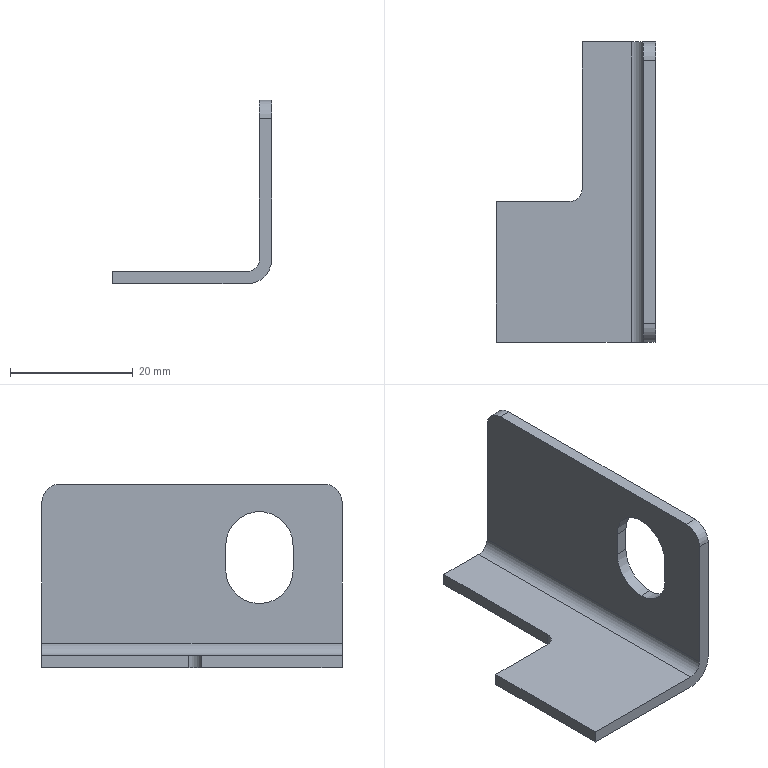Part | STEP file | 750038334 | 1 solid | 20 faces | box 26 x 49 x 30 mm | volume 4154 mm3 | plane 12 | cylinder 8 | commonest cylinder face diameters 11 x3 4 x2 6 x2 8 x1
STEP:
#1=CARTESIAN_POINT('',(24.,71.5,10.5));
#2=VERTEX_POINT('',#1);
#3=CARTESIAN_POINT('',(24.,77.,16.));
#4=VERTEX_POINT('',#3);
#5=CARTESIAN_POINT('',(24.,71.5,16.));
#6=DIRECTION('',(1.,0.,0.));
#7=DIRECTION('',(0.,0.,-1.));
#8=AXIS2_PLACEMENT_3D('',#5,#6,#7);
#9=CIRCLE('',#8,5.5);
#10=EDGE_CURVE('',#2,#4,#9,.T.);
#11=ORIENTED_EDGE('',*,*,#10,.F.);
#12=CARTESIAN_POINT('',(26.,71.5,10.5));
#13=VERTEX_POINT('',#12);
#14=CARTESIAN_POINT('',(-37.063,71.5,10.5));
#15=DIRECTION('',(1.,0.,0.));
#16=VECTOR('',#15,1000.);
#17=LINE('',#14,#16);
#18=EDGE_CURVE('',#2,#13,#17,.T.);
#19=ORIENTED_EDGE('',*,*,#18,.T.);
#20=CARTESIAN_POINT('',(26.,77.,16.));
#21=VERTEX_POINT('',#20);
#22=CARTESIAN_POINT('',(26.,71.5,16.));
#23=DIRECTION('',(-1.,0.,0.));
#24=DIRECTION('',(0.,0.,-1.));
#25=AXIS2_PLACEMENT_3D('',#22,#23,#24);
#26=CIRCLE('',#25,5.5);
#27=EDGE_CURVE('',#21,#13,#26,.T.);
#28=ORIENTED_EDGE('',*,*,#27,.F.);
#29=CARTESIAN_POINT('',(-37.063,77.,16.));
#30=DIRECTION('',(-1.,0.,0.));
#31=VECTOR('',#30,1000.);
#32=LINE('',#29,#31);
#33=EDGE_CURVE('',#21,#4,#32,.T.);
#34=ORIENTED_EDGE('',*,*,#33,.T.);
#35=EDGE_LOOP('',(#11,#19,#28,#34));
#36=FACE_OUTER_BOUND('',#35,.T.);
#37=CARTESIAN_POINT('',(-37.063,71.5,16.));
#38=DIRECTION('',(1.,0.,0.));
#39=DIRECTION('',(0.,0.,-1.));
#40=AXIS2_PLACEMENT_3D('',#37,#38,#39);
#41=CYLINDRICAL_SURFACE('',#40,5.5);
#42=ADVANCED_FACE('',(#36),#41,.F.);
#43=CARTESIAN_POINT('',(24.,107.,27.));
#44=VERTEX_POINT('',#43);
#45=CARTESIAN_POINT('',(24.,107.,4.));
#46=VERTEX_POINT('',#45);
#47=CARTESIAN_POINT('',(24.,107.,4.));
#48=DIRECTION('',(0.,0.,-1.));
#49=VECTOR('',#48,1000.);
#50=LINE('',#47,#49);
#51=EDGE_CURVE('',#44,#46,#50,.T.);
#52=ORIENTED_EDGE('',*,*,#51,.T.);
#53=CARTESIAN_POINT('',(24.,58.,4.));
#54=VERTEX_POINT('',#53);
#55=CARTESIAN_POINT('',(24.,58.,4.));
#56=DIRECTION('',(0.,-1.,0.));
#57=VECTOR('',#56,1000.);
#58=LINE('',#55,#57);
#59=EDGE_CURVE('',#46,#54,#58,.T.);
#60=ORIENTED_EDGE('',*,*,#59,.T.);
#61=CARTESIAN_POINT('',(24.,58.,27.));
#62=VERTEX_POINT('',#61);
#63=CARTESIAN_POINT('',(24.,58.,4.));
#64=DIRECTION('',(0.,0.,1.));
#65=VECTOR('',#64,1000.);
#66=LINE('',#63,#65);
#67=EDGE_CURVE('',#54,#62,#66,.T.);
#68=ORIENTED_EDGE('',*,*,#67,.T.);
#69=CARTESIAN_POINT('',(24.,61.,30.));
#70=VERTEX_POINT('',#69);
#71=CARTESIAN_POINT('',(24.,61.,27.));
#72=DIRECTION('',(-1.,0.,0.));
#73=DIRECTION('',(0.,1.,0.));
#74=AXIS2_PLACEMENT_3D('',#71,#72,#73);
#75=CIRCLE('',#74,3.);
#76=EDGE_CURVE('',#62,#70,#75,.T.);
#77=ORIENTED_EDGE('',*,*,#76,.T.);
#78=CARTESIAN_POINT('',(24.,104.,30.));
#79=VERTEX_POINT('',#78);
#80=CARTESIAN_POINT('',(24.,58.,30.));
#81=DIRECTION('',(0.,1.,0.));
#82=VECTOR('',#81,1000.);
#83=LINE('',#80,#82);
#84=EDGE_CURVE('',#70,#79,#83,.T.);
#85=ORIENTED_EDGE('',*,*,#84,.T.);
#86=CARTESIAN_POINT('',(24.,104.,27.));
#87=DIRECTION('',(-1.,0.,0.));
#88=DIRECTION('',(0.,0.,-1.));
#89=AXIS2_PLACEMENT_3D('',#86,#87,#88);
#90=CIRCLE('',#89,3.);
#91=EDGE_CURVE('',#79,#44,#90,.T.);
#92=ORIENTED_EDGE('',*,*,#91,.T.);
#93=EDGE_LOOP('',(#52,#60,#68,#77,#85,#92));
#94=FACE_OUTER_BOUND('',#93,.T.);
#95=CARTESIAN_POINT('',(24.,66.,16.));
#96=VERTEX_POINT('',#95);
#97=CARTESIAN_POINT('',(24.,71.5,16.));
#98=DIRECTION('',(1.,0.,0.));
#99=DIRECTION('',(0.,0.,-1.));
#100=AXIS2_PLACEMENT_3D('',#97,#98,#99);
#101=CIRCLE('',#100,5.5);
#102=EDGE_CURVE('',#96,#2,#101,.T.);
#103=ORIENTED_EDGE('',*,*,#102,.T.);
#104=ORIENTED_EDGE('',*,*,#10,.T.);
#105=CARTESIAN_POINT('',(24.,77.,20.));
#106=VERTEX_POINT('',#105);
#107=CARTESIAN_POINT('',(24.,77.,4.));
#108=DIRECTION('',(0.,0.,1.));
#109=VECTOR('',#108,1000.);
#110=LINE('',#107,#109);
#111=EDGE_CURVE('',#4,#106,#110,.T.);
#112=ORIENTED_EDGE('',*,*,#111,.T.);
#113=CARTESIAN_POINT('',(24.,66.,20.));
#114=VERTEX_POINT('',#113);
#115=CARTESIAN_POINT('',(24.,71.5,20.));
#116=DIRECTION('',(1.,0.,0.));
#117=DIRECTION('',(0.,0.,-1.));
#118=AXIS2_PLACEMENT_3D('',#115,#116,#117);
#119=CIRCLE('',#118,5.5);
#120=EDGE_CURVE('',#106,#114,#119,.T.);
#121=ORIENTED_EDGE('',*,*,#120,.T.);
#122=CARTESIAN_POINT('',(24.,66.,4.));
#123=DIRECTION('',(0.,0.,-1.));
#124=VECTOR('',#123,1000.);
#125=LINE('',#122,#124);
#126=EDGE_CURVE('',#114,#96,#125,.T.);
#127=ORIENTED_EDGE('',*,*,#126,.T.);
#128=EDGE_LOOP('',(#103,#104,#112,#121,#127));
#129=FACE_BOUND('',#128,.T.);
#130=CARTESIAN_POINT('',(24.,58.,4.));
#131=DIRECTION('',(-1.,0.,0.));
#132=DIRECTION('',(0.,-1.,0.));
#133=AXIS2_PLACEMENT_3D('',#130,#131,#132);
#134=PLANE('',#133);
#135=ADVANCED_FACE('',(#94,#129),#134,.T.);
#136=CARTESIAN_POINT('',(22.,58.,2.));
#137=VERTEX_POINT('',#136);
#138=CARTESIAN_POINT('',(22.,107.,2.));
#139=VERTEX_POINT('',#138);
#140=CARTESIAN_POINT('',(22.,58.,2.));
#141=DIRECTION('',(0.,1.,0.));
#142=VECTOR('',#141,1000.);
#143=LINE('',#140,#142);
#144=EDGE_CURVE('',#137,#139,#143,.T.);
#145=ORIENTED_EDGE('',*,*,#144,.F.);
#146=CARTESIAN_POINT('',(22.,58.,4.));
#147=DIRECTION('',(0.,1.,0.));
#148=DIRECTION('',(-1.,0.,0.));
#149=AXIS2_PLACEMENT_3D('',#146,#147,#148);
#150=CIRCLE('',#149,2.);
#151=EDGE_CURVE('',#54,#137,#150,.T.);
#152=ORIENTED_EDGE('',*,*,#151,.F.);
#153=ORIENTED_EDGE('',*,*,#59,.F.);
#154=CARTESIAN_POINT('',(22.,107.,4.));
#155=DIRECTION('',(0.,-1.,0.));
#156=DIRECTION('',(-1.,0.,0.));
#157=AXIS2_PLACEMENT_3D('',#154,#155,#156);
#158=CIRCLE('',#157,2.);
#159=EDGE_CURVE('',#139,#46,#158,.T.);
#160=ORIENTED_EDGE('',*,*,#159,.F.);
#161=EDGE_LOOP('',(#145,#152,#153,#160));
#162=FACE_OUTER_BOUND('',#161,.T.);
#163=CARTESIAN_POINT('',(22.,58.,4.));
#164=DIRECTION('',(0.,1.,0.));
#165=DIRECTION('',(-1.,0.,0.));
#166=AXIS2_PLACEMENT_3D('',#163,#164,#165);
#167=CYLINDRICAL_SURFACE('',#166,2.);
#168=ADVANCED_FACE('',(#162),#167,.F.);
#169=CARTESIAN_POINT('',(14.,107.,2.));
#170=VERTEX_POINT('',#169);
#171=CARTESIAN_POINT('',(14.,107.,2.));
#172=DIRECTION('',(1.,0.,0.));
#173=VECTOR('',#172,1000.);
#174=LINE('',#171,#173);
#175=EDGE_CURVE('',#170,#139,#174,.T.);
#176=ORIENTED_EDGE('',*,*,#175,.T.);
#177=ORIENTED_EDGE('',*,*,#159,.T.);
#178=ORIENTED_EDGE('',*,*,#51,.F.);
#179=CARTESIAN_POINT('',(26.,107.,27.));
#180=VERTEX_POINT('',#179);
#181=CARTESIAN_POINT('',(14.,107.,27.));
#182=DIRECTION('',(1.,0.,0.));
#183=VECTOR('',#182,1000.);
#184=LINE('',#181,#183);
#185=EDGE_CURVE('',#44,#180,#184,.T.);
#186=ORIENTED_EDGE('',*,*,#185,.T.);
#187=CARTESIAN_POINT('',(26.,107.,4.));
#188=VERTEX_POINT('',#187);
#189=CARTESIAN_POINT('',(26.,107.,2.));
#190=DIRECTION('',(0.,0.,-1.));
#191=VECTOR('',#190,1000.);
#192=LINE('',#189,#191);
#193=EDGE_CURVE('',#180,#188,#192,.T.);
#194=ORIENTED_EDGE('',*,*,#193,.T.);
#195=CARTESIAN_POINT('',(22.,107.,0.));
#196=VERTEX_POINT('',#195);
#197=CARTESIAN_POINT('',(22.,107.,4.));
#198=DIRECTION('',(0.,1.,0.));
#199=DIRECTION('',(-1.,0.,0.));
#200=AXIS2_PLACEMENT_3D('',#197,#198,#199);
#201=CIRCLE('',#200,4.);
#202=EDGE_CURVE('',#188,#196,#201,.T.);
#203=ORIENTED_EDGE('',*,*,#202,.T.);
#204=CARTESIAN_POINT('',(14.,107.,0.));
#205=VERTEX_POINT('',#204);
#206=CARTESIAN_POINT('',(14.,107.,0.));
#207=DIRECTION('',(-1.,0.,0.));
#208=VECTOR('',#207,1000.);
#209=LINE('',#206,#208);
#210=EDGE_CURVE('',#196,#205,#209,.T.);
#211=ORIENTED_EDGE('',*,*,#210,.T.);
#212=CARTESIAN_POINT('',(14.,107.,2.));
#213=DIRECTION('',(0.,0.,1.));
#214=VECTOR('',#213,1000.);
#215=LINE('',#212,#214);
#216=EDGE_CURVE('',#205,#170,#215,.T.);
#217=ORIENTED_EDGE('',*,*,#216,.T.);
#218=EDGE_LOOP('',(#176,#177,#178,#186,#194,#203,#211,#217));
#219=FACE_OUTER_BOUND('',#218,.T.);
#220=CARTESIAN_POINT('',(14.,107.,2.));
#221=DIRECTION('',(0.,1.,0.));
#222=DIRECTION('',(0.,0.,1.));
#223=AXIS2_PLACEMENT_3D('',#220,#221,#222);
#224=PLANE('',#223);
#225=ADVANCED_FACE('',(#219),#224,.T.);
#226=CARTESIAN_POINT('',(26.,104.,30.));
#227=VERTEX_POINT('',#226);
#228=CARTESIAN_POINT('',(26.,104.,27.));
#229=DIRECTION('',(-1.,0.,0.));
#230=DIRECTION('',(0.,0.,-1.));
#231=AXIS2_PLACEMENT_3D('',#228,#229,#230);
#232=CIRCLE('',#231,3.);
#233=EDGE_CURVE('',#227,#180,#232,.T.);
#234=ORIENTED_EDGE('',*,*,#233,.T.);
#235=ORIENTED_EDGE('',*,*,#185,.F.);
#236=ORIENTED_EDGE('',*,*,#91,.F.);
#237=CARTESIAN_POINT('',(14.,104.,30.));
#238=DIRECTION('',(1.,0.,0.));
#239=VECTOR('',#238,1000.);
#240=LINE('',#237,#239);
#241=EDGE_CURVE('',#79,#227,#240,.T.);
#242=ORIENTED_EDGE('',*,*,#241,.T.);
#243=EDGE_LOOP('',(#234,#235,#236,#242));
#244=FACE_OUTER_BOUND('',#243,.T.);
#245=CARTESIAN_POINT('',(14.,104.,27.));
#246=DIRECTION('',(1.,0.,0.));
#247=DIRECTION('',(0.,0.,-1.));
#248=AXIS2_PLACEMENT_3D('',#245,#246,#247);
#249=CYLINDRICAL_SURFACE('',#248,3.);
#250=ADVANCED_FACE('',(#244),#249,.T.);
#251=CARTESIAN_POINT('',(26.,61.,30.));
#252=VERTEX_POINT('',#251);
#253=CARTESIAN_POINT('',(26.,58.,30.));
#254=DIRECTION('',(0.,1.,0.));
#255=VECTOR('',#254,1000.);
#256=LINE('',#253,#255);
#257=EDGE_CURVE('',#252,#227,#256,.T.);
#258=ORIENTED_EDGE('',*,*,#257,.T.);
#259=ORIENTED_EDGE('',*,*,#241,.F.);
#260=ORIENTED_EDGE('',*,*,#84,.F.);
#261=CARTESIAN_POINT('',(24.,61.,30.));
#262=DIRECTION('',(1.,0.,0.));
#263=VECTOR('',#262,1000.);
#264=LINE('',#261,#263);
#265=EDGE_CURVE('',#70,#252,#264,.T.);
#266=ORIENTED_EDGE('',*,*,#265,.T.);
#267=EDGE_LOOP('',(#258,#259,#260,#266));
#268=FACE_OUTER_BOUND('',#267,.T.);
#269=CARTESIAN_POINT('',(24.,58.,30.));
#270=DIRECTION('',(0.,0.,1.));
#271=DIRECTION('',(1.,0.,0.));
#272=AXIS2_PLACEMENT_3D('',#269,#270,#271);
#273=PLANE('',#272);
#274=ADVANCED_FACE('',(#268),#273,.T.);
#275=CARTESIAN_POINT('',(26.,58.,27.));
#276=VERTEX_POINT('',#275);
#277=CARTESIAN_POINT('',(26.,61.,27.));
#278=DIRECTION('',(-1.,0.,0.));
#279=DIRECTION('',(0.,1.,0.));
#280=AXIS2_PLACEMENT_3D('',#277,#278,#279);
#281=CIRCLE('',#280,3.);
#282=EDGE_CURVE('',#276,#252,#281,.T.);
#283=ORIENTED_EDGE('',*,*,#282,.T.);
#284=ORIENTED_EDGE('',*,*,#265,.F.);
#285=ORIENTED_EDGE('',*,*,#76,.F.);
#286=CARTESIAN_POINT('',(24.,58.,27.));
#287=DIRECTION('',(1.,0.,0.));
#288=VECTOR('',#287,1000.);
#289=LINE('',#286,#288);
#290=EDGE_CURVE('',#62,#276,#289,.T.);
#291=ORIENTED_EDGE('',*,*,#290,.T.);
#292=EDGE_LOOP('',(#283,#284,#285,#291));
#293=FACE_OUTER_BOUND('',#292,.T.);
#294=CARTESIAN_POINT('',(24.,61.,27.));
#295=DIRECTION('',(1.,0.,0.));
#296=DIRECTION('',(0.,1.,0.));
#297=AXIS2_PLACEMENT_3D('',#294,#295,#296);
#298=CYLINDRICAL_SURFACE('',#297,3.);
#299=ADVANCED_FACE('',(#293),#298,.T.);
#300=CARTESIAN_POINT('',(0.,58.,0.));
#301=VERTEX_POINT('',#300);
#302=CARTESIAN_POINT('',(22.,58.,0.));
#303=VERTEX_POINT('',#302);
#304=CARTESIAN_POINT('',(22.,58.,0.));
#305=DIRECTION('',(1.,0.,0.));
#306=VECTOR('',#305,1000.);
#307=LINE('',#304,#306);
#308=EDGE_CURVE('',#301,#303,#307,.T.);
#309=ORIENTED_EDGE('',*,*,#308,.T.);
#310=CARTESIAN_POINT('',(26.,58.,4.));
#311=VERTEX_POINT('',#310);
#312=CARTESIAN_POINT('',(22.,58.,4.));
#313=DIRECTION('',(0.,-1.,0.));
#314=DIRECTION('',(-1.,0.,0.));
#315=AXIS2_PLACEMENT_3D('',#312,#313,#314);
#316=CIRCLE('',#315,4.);
#317=EDGE_CURVE('',#303,#311,#316,.T.);
#318=ORIENTED_EDGE('',*,*,#317,.T.);
#319=CARTESIAN_POINT('',(26.,58.,2.));
#320=DIRECTION('',(0.,0.,1.));
#321=VECTOR('',#320,1000.);
#322=LINE('',#319,#321);
#323=EDGE_CURVE('',#311,#276,#322,.T.);
#324=ORIENTED_EDGE('',*,*,#323,.T.);
#325=ORIENTED_EDGE('',*,*,#290,.F.);
#326=ORIENTED_EDGE('',*,*,#67,.F.);
#327=ORIENTED_EDGE('',*,*,#151,.T.);
#328=CARTESIAN_POINT('',(0.,58.,2.));
#329=VERTEX_POINT('',#328);
#330=CARTESIAN_POINT('',(22.,58.,2.));
#331=DIRECTION('',(-1.,0.,0.));
#332=VECTOR('',#331,1000.);
#333=LINE('',#330,#332);
#334=EDGE_CURVE('',#137,#329,#333,.T.);
#335=ORIENTED_EDGE('',*,*,#334,.T.);
#336=CARTESIAN_POINT('',(0.,58.,2.));
#337=DIRECTION('',(0.,0.,-1.));
#338=VECTOR('',#337,1000.);
#339=LINE('',#336,#338);
#340=EDGE_CURVE('',#329,#301,#339,.T.);
#341=ORIENTED_EDGE('',*,*,#340,.T.);
#342=EDGE_LOOP('',(#309,#318,#324,#325,#326,#327,#335,#341));
#343=FACE_OUTER_BOUND('',#342,.T.);
#344=CARTESIAN_POINT('',(22.,58.,2.));
#345=DIRECTION('',(0.,-1.,0.));
#346=DIRECTION('',(1.,0.,0.));
#347=AXIS2_PLACEMENT_3D('',#344,#345,#346);
#348=PLANE('',#347);
#349=ADVANCED_FACE('',(#343),#348,.T.);
#350=ORIENTED_EDGE('',*,*,#33,.F.);
#351=CARTESIAN_POINT('',(26.,77.,20.));
#352=VERTEX_POINT('',#351);
#353=CARTESIAN_POINT('',(26.,77.,16.));
#354=DIRECTION('',(0.,0.,-1.));
#355=VECTOR('',#354,1000.);
#356=LINE('',#353,#355);
#357=EDGE_CURVE('',#352,#21,#356,.T.);
#358=ORIENTED_EDGE('',*,*,#357,.F.);
#359=CARTESIAN_POINT('',(-37.063,77.,20.));
#360=DIRECTION('',(1.,0.,0.));
#361=VECTOR('',#360,1000.);
#362=LINE('',#359,#361);
#363=EDGE_CURVE('',#106,#352,#362,.T.);
#364=ORIENTED_EDGE('',*,*,#363,.F.);
#365=ORIENTED_EDGE('',*,*,#111,.F.);
#366=EDGE_LOOP('',(#350,#358,#364,#365));
#367=FACE_OUTER_BOUND('',#366,.T.);
#368=CARTESIAN_POINT('',(-37.063,77.,16.));
#369=DIRECTION('',(0.,1.,0.));
#370=DIRECTION('',(0.,0.,1.));
#371=AXIS2_PLACEMENT_3D('',#368,#369,#370);
#372=PLANE('',#371);
#373=ADVANCED_FACE('',(#367),#372,.F.);
#374=ORIENTED_EDGE('',*,*,#18,.F.);
#375=ORIENTED_EDGE('',*,*,#102,.F.);
#376=CARTESIAN_POINT('',(26.,66.,16.));
#377=VERTEX_POINT('',#376);
#378=CARTESIAN_POINT('',(-37.063,66.,16.));
#379=DIRECTION('',(-1.,0.,0.));
#380=VECTOR('',#379,1000.);
#381=LINE('',#378,#380);
#382=EDGE_CURVE('',#377,#96,#381,.T.);
#383=ORIENTED_EDGE('',*,*,#382,.F.);
#384=CARTESIAN_POINT('',(26.,71.5,16.));
#385=DIRECTION('',(-1.,0.,0.));
#386=DIRECTION('',(0.,0.,-1.));
#387=AXIS2_PLACEMENT_3D('',#384,#385,#386);
#388=CIRCLE('',#387,5.5);
#389=EDGE_CURVE('',#13,#377,#388,.T.);
#390=ORIENTED_EDGE('',*,*,#389,.F.);
#391=EDGE_LOOP('',(#374,#375,#383,#390));
#392=FACE_OUTER_BOUND('',#391,.T.);
#393=CARTESIAN_POINT('',(-37.063,71.5,16.));
#394=DIRECTION('',(1.,0.,0.));
#395=DIRECTION('',(0.,0.,-1.));
#396=AXIS2_PLACEMENT_3D('',#393,#394,#395);
#397=CYLINDRICAL_SURFACE('',#396,5.5);
#398=ADVANCED_FACE('',(#392),#397,.F.);
#399=CARTESIAN_POINT('',(26.,66.,20.));
#400=VERTEX_POINT('',#399);
#401=CARTESIAN_POINT('',(-37.063,66.,20.));
#402=DIRECTION('',(-1.,0.,0.));
#403=VECTOR('',#402,1000.);
#404=LINE('',#401,#403);
#405=EDGE_CURVE('',#400,#114,#404,.T.);
#406=ORIENTED_EDGE('',*,*,#405,.F.);
#407=CARTESIAN_POINT('',(26.,66.,20.));
#408=DIRECTION('',(0.,0.,1.));
#409=VECTOR('',#408,1000.);
#410=LINE('',#407,#409);
#411=EDGE_CURVE('',#377,#400,#410,.T.);
#412=ORIENTED_EDGE('',*,*,#411,.F.);
#413=ORIENTED_EDGE('',*,*,#382,.T.);
#414=ORIENTED_EDGE('',*,*,#126,.F.);
#415=EDGE_LOOP('',(#406,#412,#413,#414));
#416=FACE_OUTER_BOUND('',#415,.T.);
#417=CARTESIAN_POINT('',(-37.063,66.,20.));
#418=DIRECTION('',(0.,-1.,0.));
#419=DIRECTION('',(0.,0.,-1.));
#420=AXIS2_PLACEMENT_3D('',#417,#418,#419);
#421=PLANE('',#420);
#422=ADVANCED_FACE('',(#416),#421,.F.);
#423=ORIENTED_EDGE('',*,*,#363,.T.);
#424=CARTESIAN_POINT('',(26.,71.5,20.));
#425=DIRECTION('',(-1.,0.,0.));
#426=DIRECTION('',(0.,0.,-1.));
#427=AXIS2_PLACEMENT_3D('',#424,#425,#426);
#428=CIRCLE('',#427,5.5);
#429=EDGE_CURVE('',#400,#352,#428,.T.);
#430=ORIENTED_EDGE('',*,*,#429,.F.);
#431=ORIENTED_EDGE('',*,*,#405,.T.);
#432=ORIENTED_EDGE('',*,*,#120,.F.);
#433=EDGE_LOOP('',(#423,#430,#431,#432));
#434=FACE_OUTER_BOUND('',#433,.T.);
#435=CARTESIAN_POINT('',(-37.063,71.5,20.));
#436=DIRECTION('',(1.,0.,0.));
#437=DIRECTION('',(0.,0.,-1.));
#438=AXIS2_PLACEMENT_3D('',#435,#436,#437);
#439=CYLINDRICAL_SURFACE('',#438,5.5);
#440=ADVANCED_FACE('',(#434),#439,.F.);
#441=ORIENTED_EDGE('',*,*,#144,.T.);
#442=ORIENTED_EDGE('',*,*,#175,.F.);
#443=CARTESIAN_POINT('',(14.,83.,2.));
#444=VERTEX_POINT('',#443);
#445=CARTESIAN_POINT('',(14.,0.,2.));
#446=DIRECTION('',(0.,1.,0.));
#447=VECTOR('',#446,1000.);
#448=LINE('',#445,#447);
#449=EDGE_CURVE('',#444,#170,#448,.T.);
#450=ORIENTED_EDGE('',*,*,#449,.F.);
#451=CARTESIAN_POINT('',(12.,81.,2.));
#452=VERTEX_POINT('',#451);
#453=CARTESIAN_POINT('',(12.,83.,2.));
#454=DIRECTION('',(0.,0.,1.));
#455=DIRECTION('',(1.,0.,0.));
#456=AXIS2_PLACEMENT_3D('',#453,#454,#455);
#457=CIRCLE('',#456,2.);
#458=EDGE_CURVE('',#452,#444,#457,.T.);
#459=ORIENTED_EDGE('',*,*,#458,.F.);
#460=CARTESIAN_POINT('',(0.,81.,2.));
#461=VERTEX_POINT('',#460);
#462=CARTESIAN_POINT('',(0.,81.,2.));
#463=DIRECTION('',(1.,0.,0.));
#464=VECTOR('',#463,1000.);
#465=LINE('',#462,#464);
#466=EDGE_CURVE('',#461,#452,#465,.T.);
#467=ORIENTED_EDGE('',*,*,#466,.F.);
#468=CARTESIAN_POINT('',(0.,0.,2.));
#469=DIRECTION('',(0.,1.,0.));
#470=VECTOR('',#469,1000.);
#471=LINE('',#468,#470);
#472=EDGE_CURVE('',#329,#461,#471,.T.);
#473=ORIENTED_EDGE('',*,*,#472,.F.);
#474=ORIENTED_EDGE('',*,*,#334,.F.);
#475=EDGE_LOOP('',(#441,#442,#450,#459,#467,#473,#474));
#476=FACE_OUTER_BOUND('',#475,.T.);
#477=CARTESIAN_POINT('',(0.,0.,2.));
#478=DIRECTION('',(0.,0.,-1.));
#479=DIRECTION('',(-1.,0.,0.));
#480=AXIS2_PLACEMENT_3D('',#477,#478,#479);
#481=PLANE('',#480);
#482=ADVANCED_FACE('',(#476),#481,.F.);
#483=ORIENTED_EDGE('',*,*,#449,.T.);
#484=ORIENTED_EDGE('',*,*,#216,.F.);
#485=CARTESIAN_POINT('',(14.,83.,0.));
#486=VERTEX_POINT('',#485);
#487=CARTESIAN_POINT('',(14.,81.,0.));
#488=DIRECTION('',(0.,-1.,0.));
#489=VECTOR('',#488,1000.);
#490=LINE('',#487,#489);
#491=EDGE_CURVE('',#205,#486,#490,.T.);
#492=ORIENTED_EDGE('',*,*,#491,.T.);
#493=CARTESIAN_POINT('',(14.,83.,2.));
#494=DIRECTION('',(0.,0.,1.));
#495=VECTOR('',#494,1000.);
#496=LINE('',#493,#495);
#497=EDGE_CURVE('',#486,#444,#496,.T.);
#498=ORIENTED_EDGE('',*,*,#497,.T.);
#499=EDGE_LOOP('',(#483,#484,#492,#498));
#500=FACE_OUTER_BOUND('',#499,.T.);
#501=CARTESIAN_POINT('',(14.,81.,2.));
#502=DIRECTION('',(-1.,0.,0.));
#503=DIRECTION('',(0.,-1.,0.));
#504=AXIS2_PLACEMENT_3D('',#501,#502,#503);
#505=PLANE('',#504);
#506=ADVANCED_FACE('',(#500),#505,.T.);
#507=ORIENTED_EDGE('',*,*,#210,.F.);
#508=CARTESIAN_POINT('',(22.,0.,0.));
#509=DIRECTION('',(0.,-1.,0.));
#510=VECTOR('',#509,1000.);
#511=LINE('',#508,#510);
#512=EDGE_CURVE('',#196,#303,#511,.T.);
#513=ORIENTED_EDGE('',*,*,#512,.T.);
#514=ORIENTED_EDGE('',*,*,#308,.F.);
#515=CARTESIAN_POINT('',(0.,81.,0.));
#516=VERTEX_POINT('',#515);
#517=CARTESIAN_POINT('',(0.,0.,0.));
#518=DIRECTION('',(0.,1.,0.));
#519=VECTOR('',#518,1000.);
#520=LINE('',#517,#519);
#521=EDGE_CURVE('',#301,#516,#520,.T.);
#522=ORIENTED_EDGE('',*,*,#521,.T.);
#523=CARTESIAN_POINT('',(12.,81.,0.));
#524=VERTEX_POINT('',#523);
#525=CARTESIAN_POINT('',(0.,81.,0.));
#526=DIRECTION('',(1.,0.,0.));
#527=VECTOR('',#526,1000.);
#528=LINE('',#525,#527);
#529=EDGE_CURVE('',#516,#524,#528,.T.);
#530=ORIENTED_EDGE('',*,*,#529,.T.);
#531=CARTESIAN_POINT('',(12.,83.,0.));
#532=DIRECTION('',(0.,0.,1.));
#533=DIRECTION('',(1.,0.,0.));
#534=AXIS2_PLACEMENT_3D('',#531,#532,#533);
#535=CIRCLE('',#534,2.);
#536=EDGE_CURVE('',#524,#486,#535,.T.);
#537=ORIENTED_EDGE('',*,*,#536,.T.);
#538=ORIENTED_EDGE('',*,*,#491,.F.);
#539=EDGE_LOOP('',(#507,#513,#514,#522,#530,#537,#538));
#540=FACE_OUTER_BOUND('',#539,.T.);
#541=CARTESIAN_POINT('',(0.,0.,0.));
#542=DIRECTION('',(0.,0.,-1.));
#543=DIRECTION('',(-1.,0.,0.));
#544=AXIS2_PLACEMENT_3D('',#541,#542,#543);
#545=PLANE('',#544);
#546=ADVANCED_FACE('',(#540),#545,.T.);
#547=ORIENTED_EDGE('',*,*,#317,.F.);
#548=ORIENTED_EDGE('',*,*,#512,.F.);
#549=ORIENTED_EDGE('',*,*,#202,.F.);
#550=CARTESIAN_POINT('',(26.,58.,4.));
#551=DIRECTION('',(0.,-1.,0.));
#552=VECTOR('',#551,1000.);
#553=LINE('',#550,#552);
#554=EDGE_CURVE('',#188,#311,#553,.T.);
#555=ORIENTED_EDGE('',*,*,#554,.T.);
#556=EDGE_LOOP('',(#547,#548,#549,#555));
#557=FACE_OUTER_BOUND('',#556,.T.);
#558=CARTESIAN_POINT('',(22.,58.,4.));
#559=DIRECTION('',(0.,1.,0.));
#560=DIRECTION('',(-1.,0.,0.));
#561=AXIS2_PLACEMENT_3D('',#558,#559,#560);
#562=CYLINDRICAL_SURFACE('',#561,4.);
#563=ADVANCED_FACE('',(#557),#562,.T.);
#564=ORIENTED_EDGE('',*,*,#282,.F.);
#565=ORIENTED_EDGE('',*,*,#323,.F.);
#566=ORIENTED_EDGE('',*,*,#554,.F.);
#567=ORIENTED_EDGE('',*,*,#193,.F.);
#568=ORIENTED_EDGE('',*,*,#233,.F.);
#569=ORIENTED_EDGE('',*,*,#257,.F.);
#570=EDGE_LOOP('',(#564,#565,#566,#567,#568,#569));
#571=FACE_OUTER_BOUND('',#570,.T.);
#572=ORIENTED_EDGE('',*,*,#429,.T.);
#573=ORIENTED_EDGE('',*,*,#357,.T.);
#574=ORIENTED_EDGE('',*,*,#27,.T.);
#575=ORIENTED_EDGE('',*,*,#389,.T.);
#576=ORIENTED_EDGE('',*,*,#411,.T.);
#577=EDGE_LOOP('',(#572,#573,#574,#575,#576));
#578=FACE_BOUND('',#577,.T.);
#579=CARTESIAN_POINT('',(26.,58.,4.));
#580=DIRECTION('',(-1.,0.,0.));
#581=DIRECTION('',(0.,-1.,0.));
#582=AXIS2_PLACEMENT_3D('',#579,#580,#581);
#583=PLANE('',#582);
#584=ADVANCED_FACE('',(#571,#578),#583,.F.);
#585=ORIENTED_EDGE('',*,*,#472,.T.);
#586=CARTESIAN_POINT('',(0.,81.,2.));
#587=DIRECTION('',(0.,0.,-1.));
#588=VECTOR('',#587,1000.);
#589=LINE('',#586,#588);
#590=EDGE_CURVE('',#461,#516,#589,.T.);
#591=ORIENTED_EDGE('',*,*,#590,.T.);
#592=ORIENTED_EDGE('',*,*,#521,.F.);
#593=ORIENTED_EDGE('',*,*,#340,.F.);
#594=EDGE_LOOP('',(#585,#591,#592,#593));
#595=FACE_OUTER_BOUND('',#594,.T.);
#596=CARTESIAN_POINT('',(0.,58.,2.));
#597=DIRECTION('',(-1.,0.,0.));
#598=DIRECTION('',(0.,0.,1.));
#599=AXIS2_PLACEMENT_3D('',#596,#597,#598);
#600=PLANE('',#599);
#601=ADVANCED_FACE('',(#595),#600,.T.);
#602=ORIENTED_EDGE('',*,*,#497,.F.);
#603=ORIENTED_EDGE('',*,*,#536,.F.);
#604=CARTESIAN_POINT('',(12.,81.,2.));
#605=DIRECTION('',(0.,0.,-1.));
#606=VECTOR('',#605,1000.);
#607=LINE('',#604,#606);
#608=EDGE_CURVE('',#452,#524,#607,.T.);
#609=ORIENTED_EDGE('',*,*,#608,.F.);
#610=ORIENTED_EDGE('',*,*,#458,.T.);
#611=EDGE_LOOP('',(#602,#603,#609,#610));
#612=FACE_OUTER_BOUND('',#611,.T.);
#613=CARTESIAN_POINT('',(12.,83.,2.));
#614=DIRECTION('',(0.,0.,1.));
#615=DIRECTION('',(1.,0.,0.));
#616=AXIS2_PLACEMENT_3D('',#613,#614,#615);
#617=CYLINDRICAL_SURFACE('',#616,2.);
#618=ADVANCED_FACE('',(#612),#617,.F.);
#619=ORIENTED_EDGE('',*,*,#529,.F.);
#620=ORIENTED_EDGE('',*,*,#590,.F.);
#621=ORIENTED_EDGE('',*,*,#466,.T.);
#622=ORIENTED_EDGE('',*,*,#608,.T.);
#623=EDGE_LOOP('',(#619,#620,#621,#622));
#624=FACE_OUTER_BOUND('',#623,.T.);
#625=CARTESIAN_POINT('',(0.,81.,2.));
#626=DIRECTION('',(0.,1.,0.));
#627=DIRECTION('',(0.,0.,1.));
#628=AXIS2_PLACEMENT_3D('',#625,#626,#627);
#629=PLANE('',#628);
#630=ADVANCED_FACE('',(#624),#629,.T.);
#631=CLOSED_SHELL('',(#42,#135,#168,#225,#250,#274,#299,#349,#373,#398,#422,#440,#482,#506,#546,#563,#584,#601,#618,#630));
#632=MANIFOLD_SOLID_BREP('',#631);
#633=CARTESIAN_POINT('',(0.,0.,0.));
#634=DIRECTION('',(0.,0.,1.));
#635=DIRECTION('',(1.,0.,0.));
#636=AXIS2_PLACEMENT_3D('',#633,#634,#635);
#637=(LENGTH_UNIT()NAMED_UNIT(*)SI_UNIT(.MILLI.,.METRE.));
#638=UNCERTAINTY_MEASURE_WITH_UNIT(LENGTH_MEASURE(0.00001),#637,'','');
#639=(NAMED_UNIT(*)PLANE_ANGLE_UNIT()SI_UNIT($,.RADIAN.));
#640=(NAMED_UNIT(*)SI_UNIT($,.STERADIAN.)SOLID_ANGLE_UNIT());
#641=(GEOMETRIC_REPRESENTATION_CONTEXT(3)GLOBAL_UNCERTAINTY_ASSIGNED_CONTEXT((#638))GLOBAL_UNIT_ASSIGNED_CONTEXT((#637,#639,#640))REPRESENTATION_CONTEXT('',''));
#642=ADVANCED_BREP_SHAPE_REPRESENTATION('',(#632,#636),#641);